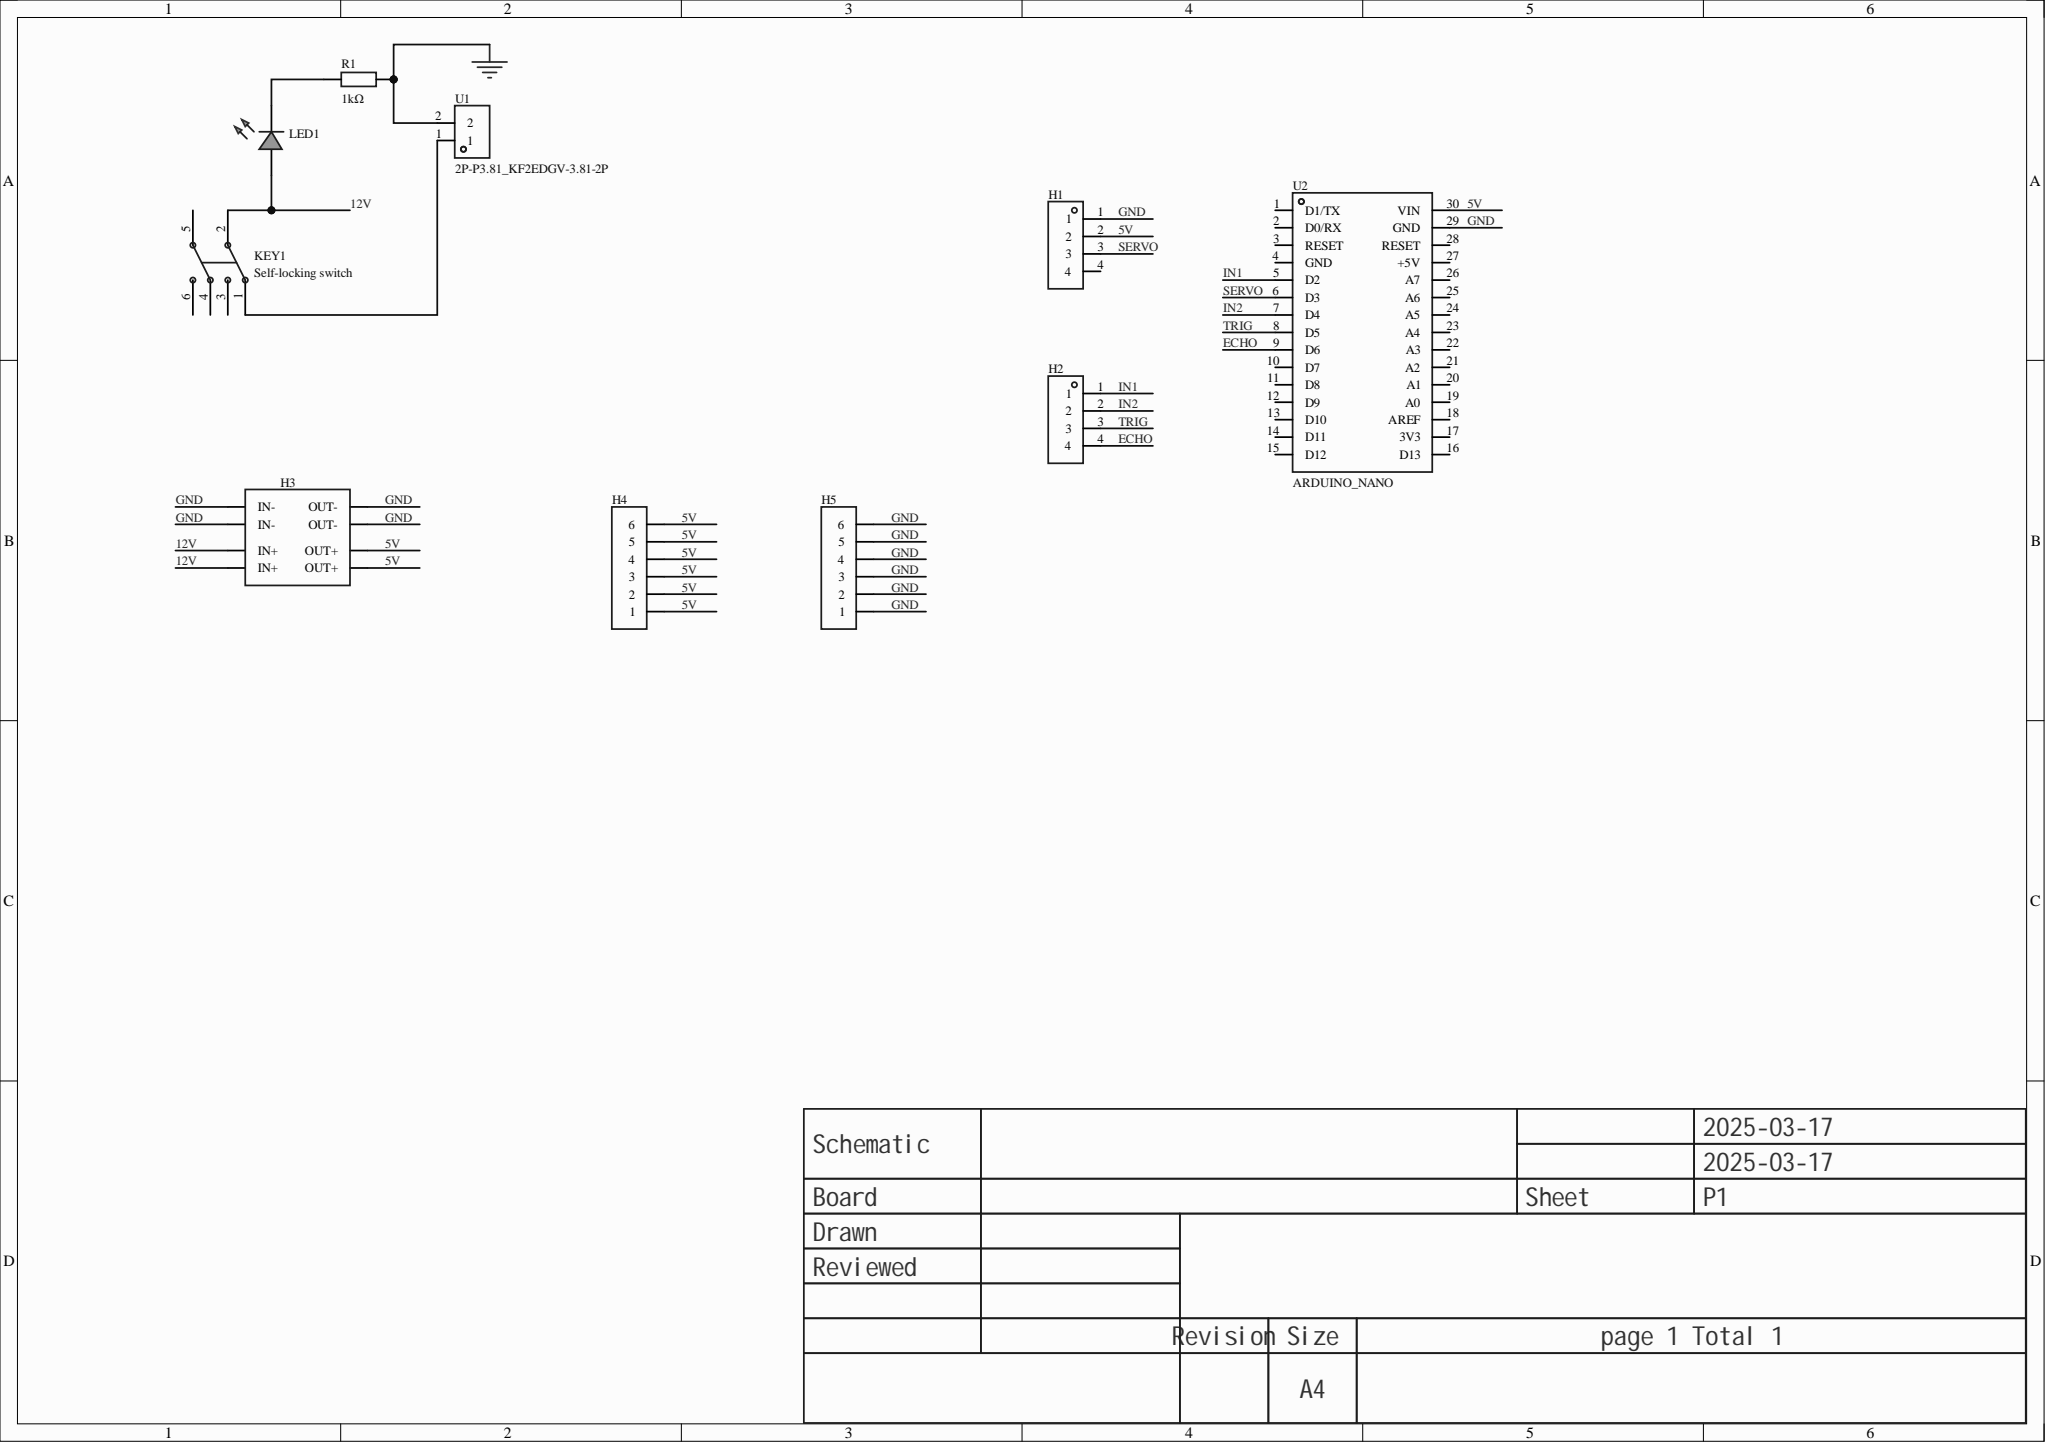Circuit board | Altium Designer | 10 parts | 10 nets
Bill of materials:
Comment,Description,Designator,Footprint,LibRef,Quantity
"","","H1, H2","HDR-TH_4P-P2.54-V-M","HDR-M_2.54_1x4P","2"
"","","H3","HDR-TH_8P-P2.54-V-M","HDR-M_2.54_1x8P","1"
"","","H4, H5","HDR-TH_6P-P2.54-V-M-1","HDR-M_2.54_1x6P","2"
"Self-locking switch","6脚，8.5×8.5","KEY1","SW-TH_6P-L8.5-W8.5-P2.54","无自锁开关 8.5×8.5 无声","1"
"","","LED1","LED_TH-3mm","LED_TH-G_3mm","1"
"1kΩ","","R1","Res_1/4W","Res_AXIAL-1/4W","1"
"2P-P3.81_KF2EDGV-3.81-2P","","U1","CONN-TH_2P-P3.81_KF2EDGV-3.81-2P","2P-P3.81_KF2EDGV-3.81-2P","1"
"ARDUINO_NANO","","U2","COMM-TH_ARDUINO_NANO","ARDUINO_NANO","1"
Netlist (Protel format):
[
H1
HDR-TH_4P-P2.54-V-M




]
[
H2
HDR-TH_4P-P2.54-V-M




]
[
H3
HDR-TH_8P-P2.54-V-M




]
[
H4
HDR-TH_6P-P2.54-V-M-1




]
[
H5
HDR-TH_6P-P2.54-V-M-1




]
[
KEY1
SW-TH_6P-L8.5-W8.5-P2.54
Self-locking switch



]
[
LED1
LED_TH-3mm




]
[
R1
Res_1/4W
1kΩ



]
[
U1
CONN-TH_2P-P3.81_KF2EDGV-3.81-2P
2P-P3.81_KF2EDGV-3.81-2P



]
[
U2
COMM-TH_ARDUINO_NANO
ARDUINO_NANO



]
(
TRIG
H2-3
U2-8
)
(
SERVO
H1-3
U2-6
)
(
NetLED1_2
LED1-2
R1-1
)
(
NetKEY1_1
KEY1-1
U1-1
)
(
IN2
H2-2
U2-7
)
(
IN1
H2-1
U2-5
)
(
GND
H1-1
H3-1
H3-2
H3-5
H3-6
H5-1
H5-2
H5-3
H5-4
H5-5
H5-6
R1-2
U1-2
U2-29
)
(
ECHO
H2-4
U2-9
)
(
12V
H3-3
H3-4
KEY1-2
LED1-1
)
(
5V
H1-2
H3-7
H3-8
H4-1
H4-2
H4-3
H4-4
H4-5
H4-6
U2-30
)